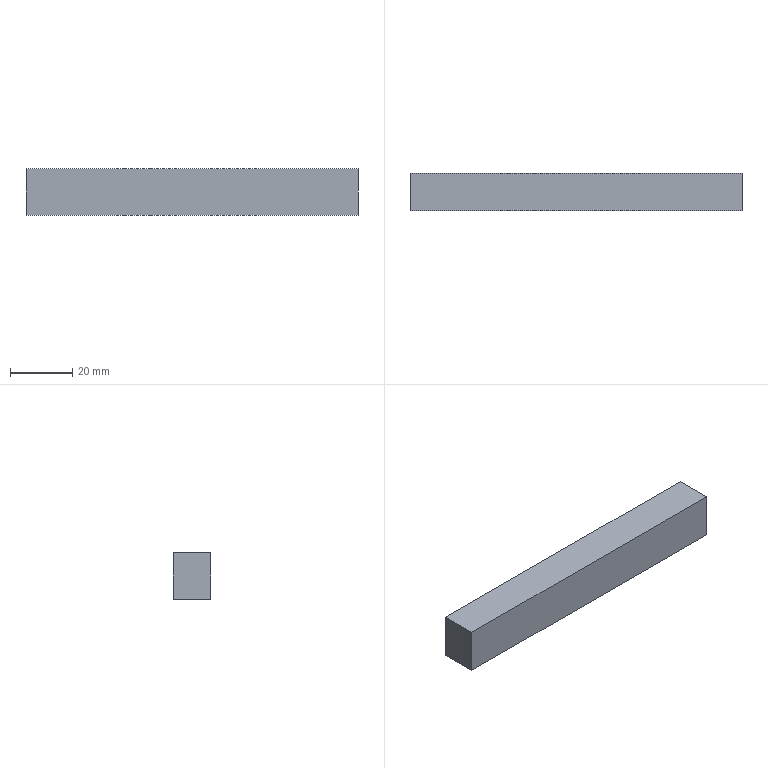Part | NX | features solid 2 | 1 solid | 6 faces | box 107 x 12 x 15 mm | volume 19260 mm3 | plane 6
STEP:
#1=CARTESIAN_POINT('',(-328.,722.,-50.));
#2=VERTEX_POINT('',#1);
#3=CARTESIAN_POINT('',(-328.,710.,-50.));
#4=VERTEX_POINT('',#3);
#5=CARTESIAN_POINT('',(-328.,741.,-50.));
#6=DIRECTION('',(0.,-1.,0.));
#7=VECTOR('',#6,1000.);
#8=LINE('',#5,#7);
#9=EDGE_CURVE('',#2,#4,#8,.T.);
#10=ORIENTED_EDGE('',*,*,#9,.F.);
#11=CARTESIAN_POINT('',(-435.,722.,-50.));
#12=VERTEX_POINT('',#11);
#13=CARTESIAN_POINT('',(-284.,722.,-50.));
#14=DIRECTION('',(-1.,0.,0.));
#15=VECTOR('',#14,1000.);
#16=LINE('',#13,#15);
#17=EDGE_CURVE('',#2,#12,#16,.T.);
#18=ORIENTED_EDGE('',*,*,#17,.T.);
#19=CARTESIAN_POINT('',(-435.,710.,-50.));
#20=VERTEX_POINT('',#19);
#21=CARTESIAN_POINT('',(-435.,800.,-50.));
#22=DIRECTION('',(0.,1.,0.));
#23=VECTOR('',#22,1000.);
#24=LINE('',#21,#23);
#25=EDGE_CURVE('',#20,#12,#24,.T.);
#26=ORIENTED_EDGE('',*,*,#25,.F.);
#27=CARTESIAN_POINT('',(-228.,710.,-50.));
#28=DIRECTION('',(-1.,0.,0.));
#29=VECTOR('',#28,1000.);
#30=LINE('',#27,#29);
#31=EDGE_CURVE('',#4,#20,#30,.T.);
#32=ORIENTED_EDGE('',*,*,#31,.F.);
#33=EDGE_LOOP('',(#10,#18,#26,#32));
#34=FACE_BOUND('',#33,.T.);
#35=CARTESIAN_POINT('',(-228.,741.,-50.));
#36=DIRECTION('',(0.,0.,1.));
#37=DIRECTION('',(0.,1.,0.));
#38=AXIS2_PLACEMENT_3D('',#35,#36,#37);
#39=PLANE('',#38);
#40=ADVANCED_FACE('',(#34),#39,.T.);
#41=CARTESIAN_POINT('',(-435.,710.,-65.));
#42=VERTEX_POINT('',#41);
#43=CARTESIAN_POINT('',(-435.,722.,-65.));
#44=VERTEX_POINT('',#43);
#45=CARTESIAN_POINT('',(-435.,800.,-65.));
#46=DIRECTION('',(0.,1.,0.));
#47=VECTOR('',#46,1000.);
#48=LINE('',#45,#47);
#49=EDGE_CURVE('',#42,#44,#48,.T.);
#50=ORIENTED_EDGE('',*,*,#49,.T.);
#51=CARTESIAN_POINT('',(-328.,722.,-65.));
#52=VERTEX_POINT('',#51);
#53=CARTESIAN_POINT('',(-284.,722.,-65.));
#54=DIRECTION('',(1.,0.,0.));
#55=VECTOR('',#54,1000.);
#56=LINE('',#53,#55);
#57=EDGE_CURVE('',#44,#52,#56,.T.);
#58=ORIENTED_EDGE('',*,*,#57,.T.);
#59=CARTESIAN_POINT('',(-328.,710.,-65.));
#60=VERTEX_POINT('',#59);
#61=CARTESIAN_POINT('',(-328.,741.,-65.));
#62=DIRECTION('',(0.,-1.,0.));
#63=VECTOR('',#62,1000.);
#64=LINE('',#61,#63);
#65=EDGE_CURVE('',#52,#60,#64,.T.);
#66=ORIENTED_EDGE('',*,*,#65,.T.);
#67=CARTESIAN_POINT('',(-284.,710.,-65.));
#68=DIRECTION('',(1.,0.,0.));
#69=VECTOR('',#68,1000.);
#70=LINE('',#67,#69);
#71=EDGE_CURVE('',#42,#60,#70,.T.);
#72=ORIENTED_EDGE('',*,*,#71,.F.);
#73=EDGE_LOOP('',(#50,#58,#66,#72));
#74=FACE_BOUND('',#73,.T.);
#75=CARTESIAN_POINT('',(-228.,741.,-65.));
#76=DIRECTION('',(0.,0.,1.));
#77=DIRECTION('',(0.,1.,0.));
#78=AXIS2_PLACEMENT_3D('',#75,#76,#77);
#79=PLANE('',#78);
#80=ADVANCED_FACE('',(#74),#79,.F.);
#81=CARTESIAN_POINT('',(-435.,710.,24.523));
#82=DIRECTION('',(0.,0.,1.));
#83=VECTOR('',#82,1000.);
#84=LINE('',#81,#83);
#85=EDGE_CURVE('',#42,#20,#84,.T.);
#86=ORIENTED_EDGE('',*,*,#85,.T.);
#87=ORIENTED_EDGE('',*,*,#25,.T.);
#88=CARTESIAN_POINT('',(-435.,722.,24.523));
#89=DIRECTION('',(0.,0.,-1.));
#90=VECTOR('',#89,1000.);
#91=LINE('',#88,#90);
#92=EDGE_CURVE('',#12,#44,#91,.T.);
#93=ORIENTED_EDGE('',*,*,#92,.T.);
#94=ORIENTED_EDGE('',*,*,#49,.F.);
#95=EDGE_LOOP('',(#86,#87,#93,#94));
#96=FACE_BOUND('',#95,.T.);
#97=CARTESIAN_POINT('',(-435.,800.,24.523));
#98=DIRECTION('',(1.,0.,0.));
#99=DIRECTION('',(0.,-1.,0.));
#100=AXIS2_PLACEMENT_3D('',#97,#98,#99);
#101=PLANE('',#100);
#102=ADVANCED_FACE('',(#96),#101,.F.);
#103=ORIENTED_EDGE('',*,*,#71,.T.);
#104=CARTESIAN_POINT('',(-328.,710.,-50.));
#105=DIRECTION('',(0.,0.,1.));
#106=VECTOR('',#105,1000.);
#107=LINE('',#104,#106);
#108=EDGE_CURVE('',#60,#4,#107,.T.);
#109=ORIENTED_EDGE('',*,*,#108,.T.);
#110=ORIENTED_EDGE('',*,*,#31,.T.);
#111=ORIENTED_EDGE('',*,*,#85,.F.);
#112=EDGE_LOOP('',(#103,#109,#110,#111));
#113=FACE_BOUND('',#112,.T.);
#114=CARTESIAN_POINT('',(-284.,710.,24.523));
#115=DIRECTION('',(0.,-1.,0.));
#116=DIRECTION('',(-1.,0.,0.));
#117=AXIS2_PLACEMENT_3D('',#114,#115,#116);
#118=PLANE('',#117);
#119=ADVANCED_FACE('',(#113),#118,.T.);
#120=ORIENTED_EDGE('',*,*,#57,.F.);
#121=ORIENTED_EDGE('',*,*,#92,.F.);
#122=ORIENTED_EDGE('',*,*,#17,.F.);
#123=CARTESIAN_POINT('',(-328.,722.,-50.));
#124=DIRECTION('',(0.,0.,1.));
#125=VECTOR('',#124,1000.);
#126=LINE('',#123,#125);
#127=EDGE_CURVE('',#52,#2,#126,.T.);
#128=ORIENTED_EDGE('',*,*,#127,.F.);
#129=EDGE_LOOP('',(#120,#121,#122,#128));
#130=FACE_BOUND('',#129,.T.);
#131=CARTESIAN_POINT('',(-284.,722.,24.523));
#132=DIRECTION('',(0.,-1.,0.));
#133=DIRECTION('',(-1.,0.,0.));
#134=AXIS2_PLACEMENT_3D('',#131,#132,#133);
#135=PLANE('',#134);
#136=ADVANCED_FACE('',(#130),#135,.F.);
#137=ORIENTED_EDGE('',*,*,#65,.F.);
#138=ORIENTED_EDGE('',*,*,#127,.T.);
#139=ORIENTED_EDGE('',*,*,#9,.T.);
#140=ORIENTED_EDGE('',*,*,#108,.F.);
#141=EDGE_LOOP('',(#137,#138,#139,#140));
#142=FACE_BOUND('',#141,.T.);
#143=CARTESIAN_POINT('',(-328.,722.,-50.));
#144=DIRECTION('',(1.,0.,0.));
#145=DIRECTION('',(0.,0.,1.));
#146=AXIS2_PLACEMENT_3D('',#143,#144,#145);
#147=PLANE('',#146);
#148=ADVANCED_FACE('',(#142),#147,.T.);
#149=CLOSED_SHELL('',(#40,#80,#102,#119,#136,#148));
#150=MANIFOLD_SOLID_BREP('',#149);
#151=(LENGTH_UNIT()NAMED_UNIT(*)SI_UNIT(.MILLI.,.METRE.));
#152=UNCERTAINTY_MEASURE_WITH_UNIT(LENGTH_MEASURE(0.00001),#151,'','');
#153=(NAMED_UNIT(*)PLANE_ANGLE_UNIT()SI_UNIT($,.RADIAN.));
#154=(NAMED_UNIT(*)SI_UNIT($,.STERADIAN.)SOLID_ANGLE_UNIT());
#155=(GEOMETRIC_REPRESENTATION_CONTEXT(3)GLOBAL_UNCERTAINTY_ASSIGNED_CONTEXT((#152))GLOBAL_UNIT_ASSIGNED_CONTEXT((#151,#153,#154))REPRESENTATION_CONTEXT('',''));
#156=ADVANCED_BREP_SHAPE_REPRESENTATION('',(#150),#155);